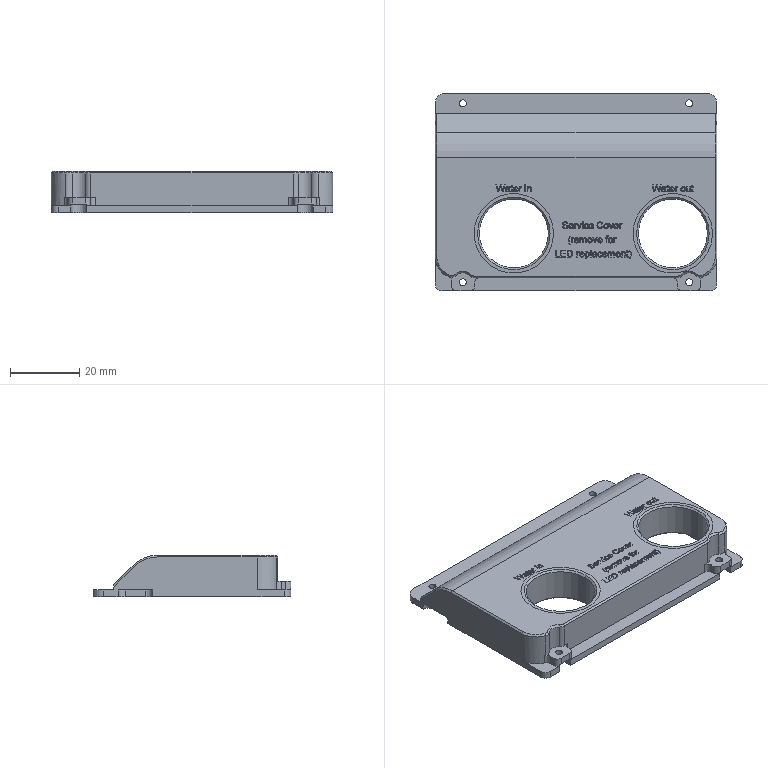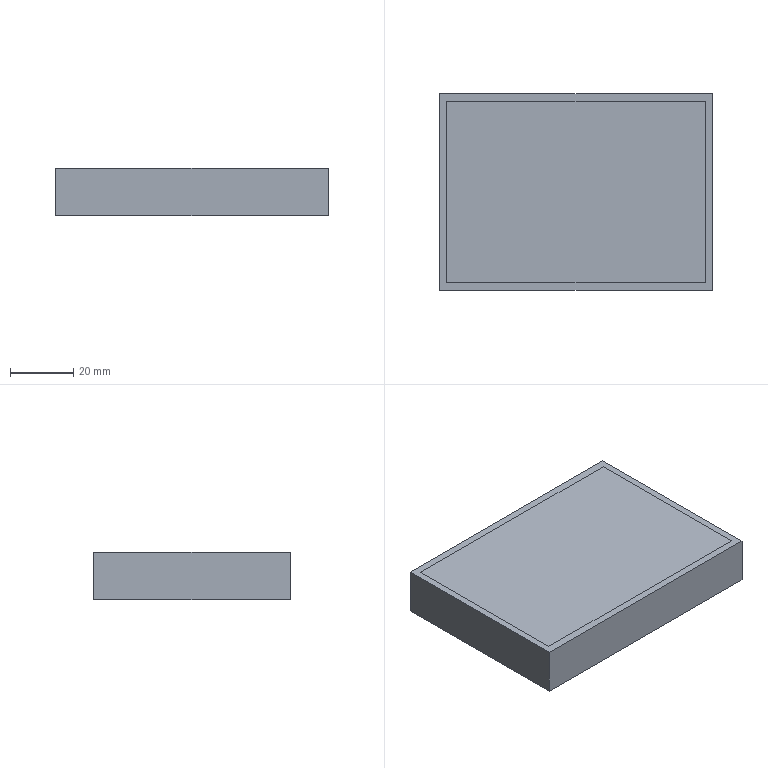CAM job | NX | 3+2 milling, drilling | part box 81.5 x 57.25 x 12.01 mm | stock box 86 x 62 x 15 mm
Tools:
number,name,description,diameter,corner_radius,flute_length,length,flutes
1,D63面刀,D63面刀,63.0,0.0,30.0,30.0,4
2,D8-25-D8-60-3T-ROUGH,D8-25-D8-60-3T-粗,8.0,0.0,25.0,60.0,2
3,点孔D4-55-90度,点孔D4-55-90度,4.0,0.0,0.0,55.0,2
5,D10R1.,Milling Tool-5 Parameters,10.0,1.0,50.0,75.0,2
7,D3-12-D4-50-3T-ROUGH,D4-12-D4-50-3T-粗,3.0,0.0,12.0,50.0,2
9,D8-25-D8-60-3T-FINISH,D8-25-D8-60-3T,8.0,0.0,25.0,60.0,3
6,D2,Milling Tool-Ball Mill,2.0,1.0,50.0,75.0,2
10,D3-12-D4-50-3T-FINISH,D4-12-D4-50-3T,3.0,0.0,12.0,50.0,3
12,D2-6-D4-50-3T-ROUGH,D2-6-D4-50-3T-粗,2.0,0.0,6.0,7.0,2
13,D2.3钻头,Drilling Tool,2.3,0.0,35.0,50.0,2
14,M2.5,Drilling Tool,2.5,0.0,35.0,50.0,4
8,D3,Milling Tool-Ball Mill,3.0,1.5,50.0,75.0,2
11,D2.3,Milling Tool-5 Parameters,2.3,0.0,50.0,75.0,2
Operations:
program,operation,operation_type,tool,method,geometry_group,spindle_rpm,surface_speed,feed_per_tooth,feed_cut,feed_plunge,cut_length_mm,path_length_mm,cut_time_min,machine_time_min
A1,FLOOR_WALL,VolumeBased25DMillingOperation,D63面刀,METHOD,WORKPIECE_54,4500.0,890.0,0.0556,2000.0,100.0,170.5,264.379,0.0852,0.0946
A1,FLOOR_WALL_COPY,VolumeBased25DMillingOperation,D63面刀,METHOD,WORKPIECE_54,4500.0,890.0,0.0278,500.0,100.0,175.0,268.979,0.35,0.3594
A1,动态粗,CavityMilling,D8-25-D8-60-3T-ROUGH,METHOD,WORKPIECE_54,6500.0,100.0,0.1178,3000.0,100.0,5831.7,8691.257,1.93,2.216
A1,ZLEVEL_PROFILE_STEEP_1_1,ZLevelMilling,D3-12-D4-50-3T-ROUGH,METHOD,WORKPIECE_54,5500.0,69.0,0.0909,1000.0,100.0,551.342,1197.723,0.5513,0.616
A1,ZLEVEL_PROFILE_STEEP_1_COPY_2,ZLevelMilling,D3-12-D4-50-3T-ROUGH,METHOD,WORKPIECE_54,5500.0,69.0,0.0909,300.0,100.0,48.897,498.99,0.163,0.208
A1,SPOT_DRILLING,Operation,点孔D4-55-90度,METHOD,WORKPIECE_54,2000.0,31.0,0.0375,150.0,0.0,16.8,374.715,0.112,0.1478
A1,PLANAR_MILL,PlanarMilling,点孔D4-55-90度,METHOD,WORKPIECE_54,5500.0,69.0,0.1091,1200.0,100.0,165.812,262.812,0.1382,0.1479
A1,PLANAR_MILL_COPY,PlanarMilling,点孔D4-55-90度,METHOD,WORKPIECE_54,5500.0,69.0,0.1091,1200.0,100.0,143.544,387.568,0.1196,0.144
A1,PLANAR_MILL_COPY_1,PlanarMilling,点孔D4-55-90度,METHOD,WORKPIECE_54,5500.0,69.0,0.1091,1200.0,100.0,98.066,214.066,0.0817,0.0933
A1,PLANAR_MILL_COPY_1_COPY,PlanarMilling,点孔D4-55-90度,METHOD,WORKPIECE_54,5500.0,69.0,0.1091,1200.0,100.0,63.0,180.0,0.0525,0.0642
A1,PLANAR_MILL_COPY_1_COPY_COPY,PlanarMilling,点孔D4-55-90度,METHOD,WORKPIECE_54,5500.0,69.0,0.1091,1200.0,100.0,42.962,317.629,0.0358,0.0633
A1,ZLEVEL_PROFILE_STEEP,ZLevelMilling,D10R1.,METHOD,WORKPIECE_54,5500.0,172.0,0.3182,3500.0,100.0,14911.47,15036.406,4.26,4.273
A1,CURVE_DRIVE_COPY,SurfaceContour,D2,METHOD,WORKPIECE_54,5500.0,34.0,0.2273,2500.0,100.0,269.947,364.327,0.108,0.1174
A1,CURVE_DRIVE,SurfaceContour,D2,METHOD,WORKPIECE_54,5500.0,34.0,0.2273,2500.0,100.0,269.897,364.277,0.108,0.1174
A1,CAVITY_MILL_COPY,CavityMilling,D8-25-D8-60-3T-FINISH,METHOD,WORKPIECE_54,6486.0,163.0,0.0308,600.0,100.0,406.719,668.81,0.6779,0.7041
A1,PLANAR_MILL_1,PlanarMilling,D8-25-D8-60-3T-FINISH,METHOD,WORKPIECE_54,5500.0,138.0,0.0364,600.0,100.0,99.5,213.5,0.1658,0.1772
A1,PLANAR_MILL_2_COPY_1,PlanarMilling,D3-12-D4-50-3T-FINISH,METHOD,WORKPIECE_54,5500.0,69.0,0.0242,400.0,100.0,220.247,431.287,0.5506,0.5717
A1,PLANAR_MILL_2,PlanarMilling,D3-12-D4-50-3T-FINISH,METHOD,WORKPIECE_54,5500.0,69.0,0.0242,400.0,100.0,213.031,421.571,0.5326,0.5534
A1,PLANAR_MILL_2_COPY,PlanarMilling,D3-12-D4-50-3T-FINISH,METHOD,WORKPIECE_54,5500.0,69.0,0.0242,400.0,100.0,236.961,561.107,0.5924,0.6248
A1,PLANAR_MILL_2_COPY_COPY_1,PlanarMilling,D3-12-D4-50-3T-FINISH,METHOD,WORKPIECE_54,5500.0,69.0,0.0242,400.0,100.0,236.961,561.507,0.5924,0.6249
A1,PLANAR_MILL_2_COPY_COPY,PlanarMilling,D3-12-D4-50-3T-FINISH,METHOD,WORKPIECE_54,5500.0,69.0,0.0242,400.0,100.0,228.656,549.202,0.5716,0.6037
B1,FLOOR_WALL_2,VolumeBased25DMillingOperation,D8-25-D8-60-3T-ROUGH,METHOD,B-G55,1061.0,100.0,0.1178,250.0,100.0,193.6,227.4,0.7744,0.7778
B1,FLOOR_WALL_2_COPY,VolumeBased25DMillingOperation,D8-25-D8-60-3T-FINISH,METHOD,B-G55,1061.0,100.0,0.1178,250.0,100.0,193.5,227.5,0.774,0.7774
C1,FLOOR_WALL_COPY_1,VolumeBased25DMillingOperation,D63面刀,METHOD,WORKPIECE_56,4500.0,890.0,0.0556,1000.0,100.0,682.0,1299.25,0.682,0.7437
C1,FLOOR_WALL_COPY_1_COPY,VolumeBased25DMillingOperation,D63面刀,METHOD,WORKPIECE_56,4500.0,890.0,0.0556,1000.0,100.0,170.5,204.5,0.1705,0.1739
C2,ADAPTIVE_MILLING,CavityMilling,D8-25-D8-60-3T-ROUGH,METHOD,WORKPIECE_56,6500.0,163.0,0.2692,3500.0,100.0,4015.104,4129.468,1.07,1.081
C2,FLOOR_WALL_COPY_1_COPY_COPY,VolumeBased25DMillingOperation,D8-25-D8-60-3T-ROUGH,METHOD,WORKPIECE_56,4500.0,890.0,0.0556,1000.0,100.0,1272.781,1311.075,1.273,1.277
C3,ADAPTIVE_MILLING_COPY,CavityMilling,D3-12-D4-50-3T-ROUGH,METHOD,WORKPIECE_56,6500.0,61.0,0.1154,1500.0,100.0,3043.862,5002.291,1.99,2.186
C4,FLOOR_WALL_3,VolumeBased25DMillingOperation,D8-25-D8-60-3T-FINISH,METHOD,WORKPIECE_56,6500.0,163.0,0.0256,500.0,100.0,599.961,637.961,1.2,1.204
C4,FLOOR_WALL_3_COPY,VolumeBased25DMillingOperation,D8-25-D8-60-3T-FINISH,METHOD,WORKPIECE_56,6500.0,163.0,0.0256,500.0,100.0,225.507,263.507,0.451,0.4548
C5,CAVITY_MILL_1,CavityMilling,D3-12-D4-50-3T-FINISH,METHOD,WORKPIECE_56,5500.0,69.0,0.0303,500.0,100.0,666.404,723.804,1.333,1.339
C5,ZLEVEL_PROFILE_STEEP_1_COPY_1_COPY_COPY,ZLevelMilling,D3-12-D4-50-3T-FINISH,METHOD,WORKPIECE_56,5500.0,69.0,0.0303,500.0,100.0,203,261,0.406,0.4118
C5,ZLEVEL_PROFILE_STEEP_1_COPY_1_COPY_COPY_COPY,ZLevelMilling,D3-12-D4-50-3T-FINISH,METHOD,WORKPIECE_56,5500.0,69.0,0.0303,500.0,100.0,203,261,0.406,0.4118
C5,PLANAR_MILL_4,PlanarMilling,D3-12-D4-50-3T-FINISH,METHOD,WORKPIECE_56,5500.0,69.0,0.0303,500.0,100.0,154.645,310.125,0.3093,0.3248
C5,PLANAR_MILL_4_COPY,PlanarMilling,D3-12-D4-50-3T-FINISH,METHOD,WORKPIECE_56,5500.0,69.0,0.0303,500.0,100.0,27.079,199.579,0.0542,0.0714
C5,PLANAR_MILL_4_COPY_COPY,PlanarMilling,D3-12-D4-50-3T-FINISH,METHOD,WORKPIECE_56,5500.0,69.0,0.0303,500.0,100.0,52.985,295.915,0.106,0.1303
C6,SPOT_DRILLING_COPY_1,Operation,点孔D4-55-90度,METHOD,WORKPIECE_56,2000.0,31.0,0.0375,150.0,0.0,17.0,248.39,0.1133,0.1365
C6,PLANAR_MILL_COPY_2,PlanarMilling,点孔D4-55-90度,METHOD,WORKPIECE_56,5500.0,69.0,0.1091,1200.0,100.0,309.195,345.195,0.2577,0.2613
C6,PLANAR_MILL_COPY_2_COPY,PlanarMilling,点孔D4-55-90度,METHOD,WORKPIECE_56,5500.0,69.0,0.1091,1200.0,100.0,242.549,278.549,0.2021,0.2057
C6,PLANAR_MILL_COPY_2_COPY_1,PlanarMilling,点孔D4-55-90度,METHOD,WORKPIECE_56,5500.0,69.0,0.1091,1200.0,100.0,219.255,261.255,0.1827,0.1869
C6,PLANAR_MILL_COPY_2_COPY_1_COPY,PlanarMilling,点孔D4-55-90度,METHOD,WORKPIECE_56,5500.0,69.0,0.1091,1200.0,100.0,139.042,267.065,0.1159,0.1287
C6,DRILLING,Operation,D2.3钻头,METHOD,WORKPIECE_56,2500.0,18.0,0.04,200.0,0.0,36.0,307.128,0.18,0.2071
C6,DRILLING_COPY,Operation,M2.5,METHOD,WORKPIECE_56,300.0,2.0,0.0004,0.45,0.0,32.0,299.128,71.111,71.138
C7,CURVE_DRIVE_COPY_COPY_COPY_COPY,SurfaceContour,D3,METHOD,C-G56,5500.0,34.0,0.0909,1000.0,100.0,1062.639,1129.243,1.063,1.069
C7,CURVE_DRIVE_COPY_COPY_COPY,SurfaceContour,D2,METHOD,C-G56,5500.0,34.0,0.0727,800.0,100.0,869.55,903.744,1.087,1.09
C8,PLANAR_MILL_8,PlanarMilling,D2-6-D4-50-3T-ROUGH,METHOD,WORKPIECE_56,6000.0,37.0,0.0417,500.0,100.0,64.46,136.343,0.1289,0.1361
C8,HOLE_MILLING,CylinderMilling,D2-6-D4-50-3T-ROUGH,METHOD,WORKPIECE_56,4500.0,28.0,0.1111,1000.0,100.0,53.429,199.529,0.0534,0.068
C-G56,ZLEVEL_PROFILE_STEEP_1_COPY_1_COPY_1,ZLevelMilling,D2-6-D4-50-3T-ROUGH,METHOD,WORKPIECE_56,5500.0,69.0,0.0303,500.0,100.0,238.832,282.832,0.4777,0.4821
C-G56,ZLEVEL_PROFILE_STEEP_1_COPY_1_COPY_1_COPY,ZLevelMilling,D2-6-D4-50-3T-ROUGH,METHOD,WORKPIECE_56,5500.0,69.0,0.0303,500.0,100.0,238.832,282.832,0.4777,0.4821
D1,FLOOR_WALL_1,VolumeBased25DMillingOperation,D8-25-D8-60-3T-ROUGH,METHOD,WORKPIECE_57,5500.0,138.0,0.1364,600.0,100.0,172.155,333.59,0.2869,0.3031
D2,FLOOR_WALL_1_COPY,VolumeBased25DMillingOperation,D8-25-D8-60-3T-FINISH,METHOD,WORKPIECE_57,5500.0,138.0,0.0364,600.0,100.0,86.025,140.025,0.1434,0.1488
D3,PLANAR_MILL_6,PlanarMilling,D2.3,METHOD,WORKPIECE_57,5500.0,138.0,0.0364,100.0,100.0,22.614,85.853,0.2261,0.2325
D3,PLANAR_MILL_6_COPY,PlanarMilling,D2.3,METHOD,WORKPIECE_57,5500.0,138.0,0.0364,100.0,100.0,22.614,85.853,0.2261,0.2325
E1,PLANAR_MILL_7,PlanarMilling,D2.3,METHOD,WORKPIECE_58,5500.0,25.0,0.0121,200.0,100.0,37.641,71.641,0.1882,0.1916